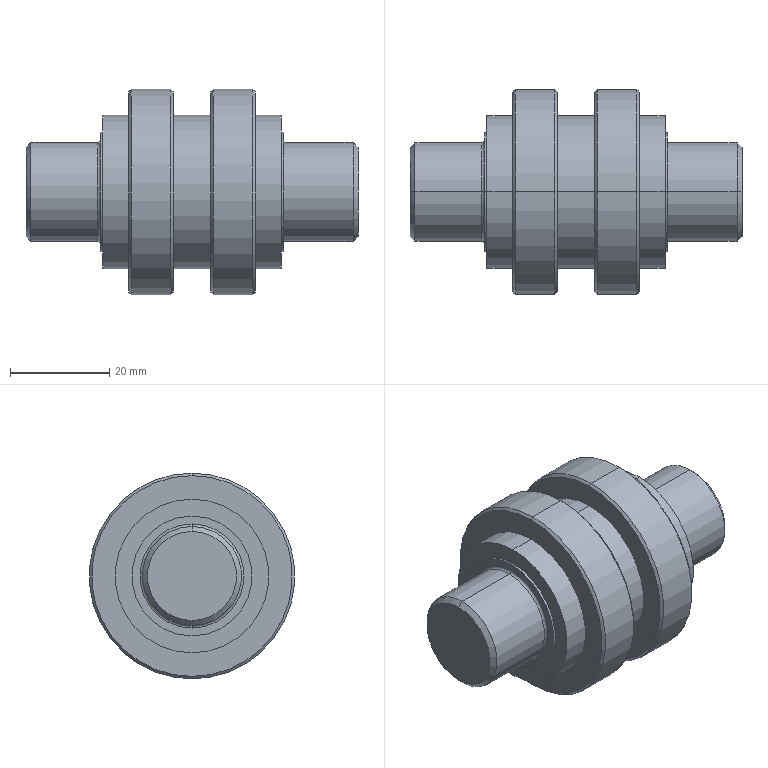Part | STEP file | 1 solid | 42 faces | box 67 x 41.5 x 41.5 mm | volume 47696 mm3 | cylinder 18 | cone 12 | plane 10 | torus 2 | commonest cylinder face diameters 31 x6 20 x4 24.2 x4 41.5 x4